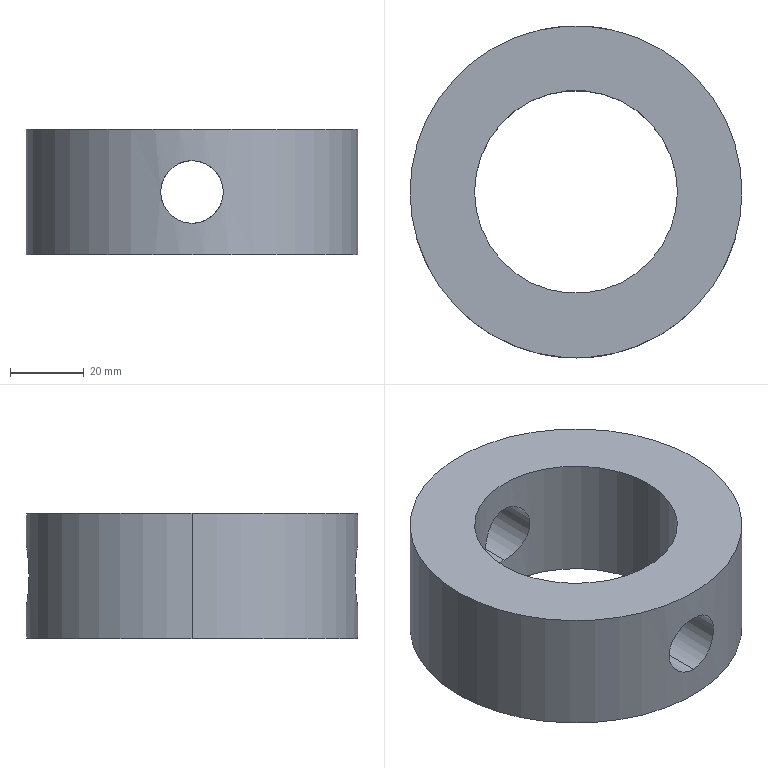Part | SolidWorks | features Extrusion 1, ICE 1 | 1 solid | 10 faces | box 90 x 90 x 34 mm | volume 127515 mm3 | cylinder 8 | plane 2 | commonest cylinder face diameters 17 x4 55 x2 90 x2
STEP:
#1=CARTESIAN_POINT('',(0.,-45.,8.5));
#2=VERTEX_POINT('',#1);
#3=CARTESIAN_POINT('',(0.,-45.,25.5));
#4=VERTEX_POINT('',#3);
#5=CARTESIAN_POINT('',(0.,-45.,8.5));
#6=CARTESIAN_POINT('',(-0.5553,-45.,8.5));
#7=CARTESIAN_POINT('',(-1.108,-44.99,8.554));
#8=CARTESIAN_POINT('',(-1.933,-44.959,8.718));
#9=CARTESIAN_POINT('',(-2.206,-44.947,8.786));
#10=CARTESIAN_POINT('',(-2.738,-44.917,8.948));
#11=CARTESIAN_POINT('',(-2.999,-44.901,9.042));
#12=CARTESIAN_POINT('',(-3.51,-44.864,9.254));
#13=CARTESIAN_POINT('',(-3.761,-44.843,9.372));
#14=CARTESIAN_POINT('',(-4.252,-44.799,9.635));
#15=CARTESIAN_POINT('',(-4.494,-44.776,9.78));
#16=CARTESIAN_POINT('',(-5.188,-44.702,10.244));
#17=CARTESIAN_POINT('',(-5.615,-44.65,10.595));
#18=CARTESIAN_POINT('',(-6.399,-44.544,11.378));
#19=CARTESIAN_POINT('',(-6.757,-44.491,11.814));
#20=CARTESIAN_POINT('',(-7.373,-44.393,12.734));
#21=CARTESIAN_POINT('',(-7.635,-44.348,13.222));
#22=CARTESIAN_POINT('',(-7.956,-44.291,13.995));
#23=CARTESIAN_POINT('',(-8.051,-44.274,14.26));
#24=CARTESIAN_POINT('',(-8.213,-44.244,14.793));
#25=CARTESIAN_POINT('',(-8.348,-44.219,15.331));
#26=CARTESIAN_POINT('',(-8.43,-44.203,15.88));
#27=CARTESIAN_POINT('',(-8.486,-44.193,16.434));
#28=CARTESIAN_POINT('',(-8.5,-44.19,16.715));
#29=CARTESIAN_POINT('',(-8.5,-44.19,17.557));
#30=CARTESIAN_POINT('',(-8.446,-44.201,18.109));
#31=CARTESIAN_POINT('',(-8.284,-44.231,18.926));
#32=CARTESIAN_POINT('',(-8.216,-44.244,19.196));
#33=CARTESIAN_POINT('',(-8.054,-44.274,19.732));
#34=CARTESIAN_POINT('',(-7.959,-44.291,19.997));
#35=CARTESIAN_POINT('',(-7.64,-44.347,20.767));
#36=CARTESIAN_POINT('',(-7.379,-44.392,21.255));
#37=CARTESIAN_POINT('',(-6.916,-44.466,21.949));
#38=CARTESIAN_POINT('',(-6.749,-44.491,22.175));
#39=CARTESIAN_POINT('',(-6.396,-44.544,22.606));
#40=CARTESIAN_POINT('',(-6.21,-44.57,22.811));
#41=CARTESIAN_POINT('',(-5.624,-44.649,23.397));
#42=CARTESIAN_POINT('',(-5.197,-44.701,23.75));
#43=CARTESIAN_POINT('',(-4.266,-44.8,24.373));
#44=CARTESIAN_POINT('',(-3.776,-44.844,24.635));
#45=CARTESIAN_POINT('',(-3.01,-44.9,24.954));
#46=CARTESIAN_POINT('',(-2.749,-44.917,25.048));
#47=CARTESIAN_POINT('',(-2.215,-44.946,25.211));
#48=CARTESIAN_POINT('',(-1.941,-44.959,25.28));
#49=CARTESIAN_POINT('',(-1.119,-44.989,25.445));
#50=CARTESIAN_POINT('',(-0.5628,-45.,25.5));
#51=CARTESIAN_POINT('',(0.,-45.,25.5));
#52=B_SPLINE_CURVE_WITH_KNOTS('',3,(#5,#6,#7,#8,#9,#10,#11,#12,#13,#14,#15,#16,#17,#18,#19,#20,#21,#22,#23,#24,#25,#26,#27,#28,#29,#30,#31,#32,#33,#34,#35,#36,#37,#38,#39,#40,#41,#42,#43,#44,#45,#46,#47,#48,#49,#50,#51),.UNSPECIFIED.,.F.,.F.,(4,2,2,2,2,2,2,2,2,2,1,2,2,2,2,2,2,2,2,2,2,2,2,4),(0.02663,0.0283,0.02913,0.02996,0.0308,0.03163,0.03329,0.03496,0.03662,0.03745,0.03828,0.03912,0.03995,0.04161,0.04245,0.04328,0.04494,0.04577,0.04661,0.04827,0.04993,0.05077,0.0516,0.05326),.UNSPECIFIED.);
#53=EDGE_CURVE('',#2,#4,#52,.T.);
#54=ORIENTED_EDGE('',*,*,#53,.F.);
#55=CARTESIAN_POINT('',(0.,-27.5,8.5));
#56=VERTEX_POINT('',#55);
#57=CARTESIAN_POINT('',(0.,-45.,8.5));
#58=DIRECTION('',(0.,1.,0.));
#59=VECTOR('',#58,1000.);
#60=LINE('',#57,#59);
#61=EDGE_CURVE('',#2,#56,#60,.T.);
#62=ORIENTED_EDGE('',*,*,#61,.T.);
#63=CARTESIAN_POINT('',(0.,-27.5,25.5));
#64=VERTEX_POINT('',#63);
#65=CARTESIAN_POINT('',(0.,-27.5,8.5));
#66=CARTESIAN_POINT('',(-0.2784,-27.5,8.5));
#67=CARTESIAN_POINT('',(-0.5567,-27.496,8.514));
#68=CARTESIAN_POINT('',(-1.113,-27.479,8.569));
#69=CARTESIAN_POINT('',(-1.392,-27.466,8.61));
#70=CARTESIAN_POINT('',(-2.219,-27.416,8.776));
#71=CARTESIAN_POINT('',(-2.751,-27.367,8.938));
#72=CARTESIAN_POINT('',(-3.776,-27.244,9.364));
#73=CARTESIAN_POINT('',(-4.273,-27.17,9.631));
#74=CARTESIAN_POINT('',(-5.192,-27.009,10.247));
#75=CARTESIAN_POINT('',(-5.618,-26.923,10.597));
#76=CARTESIAN_POINT('',(-6.206,-26.791,11.185));
#77=CARTESIAN_POINT('',(-6.394,-26.747,11.393));
#78=CARTESIAN_POINT('',(-6.746,-26.66,11.821));
#79=CARTESIAN_POINT('',(-6.91,-26.618,12.042));
#80=CARTESIAN_POINT('',(-7.37,-26.496,12.729));
#81=CARTESIAN_POINT('',(-7.633,-26.42,13.218));
#82=CARTESIAN_POINT('',(-8.063,-26.292,14.253));
#83=CARTESIAN_POINT('',(-8.225,-26.241,14.784));
#84=CARTESIAN_POINT('',(-8.389,-26.189,15.602));
#85=CARTESIAN_POINT('',(-8.43,-26.176,15.878));
#86=CARTESIAN_POINT('',(-8.486,-26.158,16.436));
#87=CARTESIAN_POINT('',(-8.5,-26.153,16.72));
#88=CARTESIAN_POINT('',(-8.5,-26.153,17.56));
#89=CARTESIAN_POINT('',(-8.445,-26.171,18.114));
#90=CARTESIAN_POINT('',(-8.281,-26.224,18.936));
#91=CARTESIAN_POINT('',(-8.212,-26.245,19.21));
#92=CARTESIAN_POINT('',(-8.049,-26.296,19.746));
#93=CARTESIAN_POINT('',(-7.955,-26.325,20.008));
#94=CARTESIAN_POINT('',(-7.636,-26.42,20.776));
#95=CARTESIAN_POINT('',(-7.374,-26.495,21.265));
#96=CARTESIAN_POINT('',(-6.753,-26.66,22.193));
#97=CARTESIAN_POINT('',(-6.402,-26.747,22.619));
#98=CARTESIAN_POINT('',(-5.818,-26.878,23.203));
#99=CARTESIAN_POINT('',(-5.613,-26.922,23.389));
#100=CARTESIAN_POINT('',(-5.184,-27.008,23.742));
#101=CARTESIAN_POINT('',(-4.959,-27.05,23.909));
#102=CARTESIAN_POINT('',(-4.269,-27.171,24.371));
#103=CARTESIAN_POINT('',(-3.782,-27.244,24.632));
#104=CARTESIAN_POINT('',(-3.013,-27.336,24.953));
#105=CARTESIAN_POINT('',(-2.749,-27.364,25.048));
#106=CARTESIAN_POINT('',(-2.212,-27.412,25.212));
#107=CARTESIAN_POINT('',(-1.941,-27.433,25.28));
#108=CARTESIAN_POINT('',(-1.121,-27.483,25.444));
#109=CARTESIAN_POINT('',(-0.5652,-27.5,25.5));
#110=CARTESIAN_POINT('',(0.,-27.5,25.5));
#111=B_SPLINE_CURVE_WITH_KNOTS('',3,(#65,#66,#67,#68,#69,#70,#71,#72,#73,#74,#75,#76,#77,#78,#79,#80,#81,#82,#83,#84,#85,#86,#87,#88,#89,#90,#91,#92,#93,#94,#95,#96,#97,#98,#99,#100,#101,#102,#103,#104,#105,#106,#107,#108,#109,#110),.UNSPECIFIED.,.F.,.F.,(4,2,2,2,2,2,2,2,2,2,2,2,2,2,2,2,2,2,2,2,2,2,4),(0.02674,0.02758,0.02841,0.03008,0.03175,0.03342,0.03426,0.03509,0.03676,0.03844,0.03927,0.04011,0.04178,0.04261,0.04345,0.04512,0.04679,0.04762,0.04846,0.05013,0.05097,0.0518,0.05347),.UNSPECIFIED.);
#112=EDGE_CURVE('',#56,#64,#111,.T.);
#113=ORIENTED_EDGE('',*,*,#112,.T.);
#114=CARTESIAN_POINT('',(0.,-45.,25.5));
#115=DIRECTION('',(0.,1.,0.));
#116=VECTOR('',#115,1000.);
#117=LINE('',#114,#116);
#118=EDGE_CURVE('',#4,#64,#117,.T.);
#119=ORIENTED_EDGE('',*,*,#118,.F.);
#120=EDGE_LOOP('',(#54,#62,#113,#119));
#121=FACE_OUTER_BOUND('',#120,.T.);
#122=CARTESIAN_POINT('',(0.,-45.,17.));
#123=DIRECTION('',(0.,1.,0.));
#124=DIRECTION('',(0.,0.,1.));
#125=AXIS2_PLACEMENT_3D('',#122,#123,#124);
#126=CYLINDRICAL_SURFACE('',#125,8.5);
#127=ADVANCED_FACE('',(#121),#126,.F.);
#128=CARTESIAN_POINT('',(0.,27.5,25.5));
#129=VERTEX_POINT('',#128);
#130=CARTESIAN_POINT('',(0.,27.5,8.5));
#131=VERTEX_POINT('',#130);
#132=CARTESIAN_POINT('',(0.,27.5,25.5));
#133=CARTESIAN_POINT('',(-0.5653,27.5,25.5));
#134=CARTESIAN_POINT('',(-1.121,27.483,25.444));
#135=CARTESIAN_POINT('',(-1.939,27.433,25.281));
#136=CARTESIAN_POINT('',(-2.209,27.412,25.213));
#137=CARTESIAN_POINT('',(-2.745,27.364,25.049));
#138=CARTESIAN_POINT('',(-3.011,27.336,24.954));
#139=CARTESIAN_POINT('',(-3.782,27.244,24.633));
#140=CARTESIAN_POINT('',(-4.269,27.171,24.371));
#141=CARTESIAN_POINT('',(-4.96,27.05,23.909));
#142=CARTESIAN_POINT('',(-5.185,27.008,23.741));
#143=CARTESIAN_POINT('',(-5.614,26.922,23.389));
#144=CARTESIAN_POINT('',(-5.818,26.878,23.203));
#145=CARTESIAN_POINT('',(-6.402,26.747,22.618));
#146=CARTESIAN_POINT('',(-6.753,26.66,22.193));
#147=CARTESIAN_POINT('',(-7.374,26.495,21.265));
#148=CARTESIAN_POINT('',(-7.635,26.42,20.776));
#149=CARTESIAN_POINT('',(-7.954,26.325,20.01));
#150=CARTESIAN_POINT('',(-8.048,26.296,19.749));
#151=CARTESIAN_POINT('',(-8.211,26.246,19.215));
#152=CARTESIAN_POINT('',(-8.28,26.224,18.94));
#153=CARTESIAN_POINT('',(-8.445,26.171,18.116));
#154=CARTESIAN_POINT('',(-8.5,26.153,17.562));
#155=CARTESIAN_POINT('',(-8.5,26.153,16.446));
#156=CARTESIAN_POINT('',(-8.444,26.172,15.878));
#157=CARTESIAN_POINT('',(-8.225,26.241,14.785));
#158=CARTESIAN_POINT('',(-8.064,26.292,14.254));
#159=CARTESIAN_POINT('',(-7.741,26.388,13.479));
#160=CARTESIAN_POINT('',(-7.621,26.423,13.225));
#161=CARTESIAN_POINT('',(-7.359,26.498,12.736));
#162=CARTESIAN_POINT('',(-7.216,26.537,12.5));
#163=CARTESIAN_POINT('',(-6.909,26.618,12.041));
#164=CARTESIAN_POINT('',(-6.744,26.661,11.819));
#165=CARTESIAN_POINT('',(-6.393,26.747,11.391));
#166=CARTESIAN_POINT('',(-6.204,26.792,11.183));
#167=CARTESIAN_POINT('',(-5.616,26.923,10.596));
#168=CARTESIAN_POINT('',(-5.191,27.01,10.246));
#169=CARTESIAN_POINT('',(-4.272,27.17,9.631));
#170=CARTESIAN_POINT('',(-3.774,27.245,9.364));
#171=CARTESIAN_POINT('',(-2.75,27.367,8.938));
#172=CARTESIAN_POINT('',(-2.22,27.416,8.776));
#173=CARTESIAN_POINT('',(-1.396,27.466,8.611));
#174=CARTESIAN_POINT('',(-1.115,27.479,8.569));
#175=CARTESIAN_POINT('',(-0.5572,27.496,8.514));
#176=CARTESIAN_POINT('',(-0.2785,27.5,8.5));
#177=CARTESIAN_POINT('',(0.,27.5,8.5));
#178=B_SPLINE_CURVE_WITH_KNOTS('',3,(#132,#133,#134,#135,#136,#137,#138,#139,#140,#141,#142,#143,#144,#145,#146,#147,#148,#149,#150,#151,#152,#153,#154,#155,#156,#157,#158,#159,#160,#161,#162,#163,#164,#165,#166,#167,#168,#169,#170,#171,#172,#173,#174,#175,#176,#177),.UNSPECIFIED.,.F.,.F.,(4,2,2,2,2,2,2,2,2,2,2,2,2,2,2,2,2,2,2,2,2,2,4),(0.,0.001671,0.002507,0.003342,0.005014,0.005849,0.006685,0.008356,0.01003,0.01086,0.0117,0.01337,0.01504,0.01671,0.01755,0.01838,0.01922,0.02005,0.02173,0.0234,0.02507,0.0259,0.02674),.UNSPECIFIED.);
#179=EDGE_CURVE('',#129,#131,#178,.T.);
#180=ORIENTED_EDGE('',*,*,#179,.T.);
#181=CARTESIAN_POINT('',(0.,45.,8.5));
#182=VERTEX_POINT('',#181);
#183=CARTESIAN_POINT('',(0.,-45.,8.5));
#184=DIRECTION('',(0.,1.,0.));
#185=VECTOR('',#184,1000.);
#186=LINE('',#183,#185);
#187=EDGE_CURVE('',#131,#182,#186,.T.);
#188=ORIENTED_EDGE('',*,*,#187,.T.);
#189=CARTESIAN_POINT('',(0.,45.,25.5));
#190=VERTEX_POINT('',#189);
#191=CARTESIAN_POINT('',(0.,45.,25.5));
#192=CARTESIAN_POINT('',(-0.563,45.,25.5));
#193=CARTESIAN_POINT('',(-1.116,44.989,25.445));
#194=CARTESIAN_POINT('',(-1.932,44.959,25.282));
#195=CARTESIAN_POINT('',(-2.202,44.947,25.215));
#196=CARTESIAN_POINT('',(-2.737,44.917,25.052));
#197=CARTESIAN_POINT('',(-3.002,44.9,24.957));
#198=CARTESIAN_POINT('',(-3.774,44.844,24.637));
#199=CARTESIAN_POINT('',(-4.262,44.8,24.375));
#200=CARTESIAN_POINT('',(-4.954,44.727,23.913));
#201=CARTESIAN_POINT('',(-5.179,44.701,23.746));
#202=CARTESIAN_POINT('',(-5.611,44.649,23.391));
#203=CARTESIAN_POINT('',(-5.816,44.623,23.205));
#204=CARTESIAN_POINT('',(-6.403,44.544,22.618));
#205=CARTESIAN_POINT('',(-6.754,44.491,22.191));
#206=CARTESIAN_POINT('',(-7.22,44.417,21.494));
#207=CARTESIAN_POINT('',(-7.365,44.393,21.253));
#208=CARTESIAN_POINT('',(-7.626,44.349,20.764));
#209=CARTESIAN_POINT('',(-7.745,44.329,20.513));
#210=CARTESIAN_POINT('',(-7.957,44.291,20.002));
#211=CARTESIAN_POINT('',(-8.051,44.274,19.741));
#212=CARTESIAN_POINT('',(-8.213,44.244,19.208));
#213=CARTESIAN_POINT('',(-8.282,44.231,18.935));
#214=CARTESIAN_POINT('',(-8.446,44.201,18.112));
#215=CARTESIAN_POINT('',(-8.5,44.19,17.559));
#216=CARTESIAN_POINT('',(-8.5,44.19,16.447));
#217=CARTESIAN_POINT('',(-8.445,44.201,15.883));
#218=CARTESIAN_POINT('',(-8.227,44.242,14.792));
#219=CARTESIAN_POINT('',(-8.066,44.272,14.261));
#220=CARTESIAN_POINT('',(-7.746,44.329,13.488));
#221=CARTESIAN_POINT('',(-7.625,44.349,13.233));
#222=CARTESIAN_POINT('',(-7.362,44.394,12.742));
#223=CARTESIAN_POINT('',(-7.219,44.417,12.505));
#224=CARTESIAN_POINT('',(-6.758,44.491,11.815));
#225=CARTESIAN_POINT('',(-6.405,44.544,11.385));
#226=CARTESIAN_POINT('',(-5.615,44.65,10.594));
#227=CARTESIAN_POINT('',(-5.187,44.702,10.243));
#228=CARTESIAN_POINT('',(-4.497,44.775,9.782));
#229=CARTESIAN_POINT('',(-4.259,44.799,9.639));
#230=CARTESIAN_POINT('',(-3.767,44.843,9.375));
#231=CARTESIAN_POINT('',(-3.513,44.863,9.255));
#232=CARTESIAN_POINT('',(-2.742,44.919,8.935));
#233=CARTESIAN_POINT('',(-2.212,44.949,8.774));
#234=CARTESIAN_POINT('',(-1.393,44.979,8.61));
#235=CARTESIAN_POINT('',(-1.114,44.987,8.569));
#236=CARTESIAN_POINT('',(-0.5561,44.997,8.514));
#237=CARTESIAN_POINT('',(-0.2777,45.,8.5));
#238=CARTESIAN_POINT('',(0.,45.,8.5));
#239=B_SPLINE_CURVE_WITH_KNOTS('',3,(#191,#192,#193,#194,#195,#196,#197,#198,#199,#200,#201,#202,#203,#204,#205,#206,#207,#208,#209,#210,#211,#212,#213,#214,#215,#216,#217,#218,#219,#220,#221,#222,#223,#224,#225,#226,#227,#228,#229,#230,#231,#232,#233,#234,#235,#236,#237,#238),.UNSPECIFIED.,.F.,.F.,(4,2,2,2,2,2,2,2,2,2,2,2,2,2,2,2,2,2,2,2,2,2,2,4),(0.,0.001665,0.002497,0.003329,0.004994,0.005826,0.006659,0.008323,0.009156,0.009988,0.01082,0.01165,0.01332,0.01498,0.01665,0.01748,0.01831,0.01998,0.02164,0.02247,0.02331,0.02497,0.0258,0.02663),.UNSPECIFIED.);
#240=EDGE_CURVE('',#190,#182,#239,.T.);
#241=ORIENTED_EDGE('',*,*,#240,.F.);
#242=CARTESIAN_POINT('',(0.,-45.,25.5));
#243=DIRECTION('',(0.,1.,0.));
#244=VECTOR('',#243,1000.);
#245=LINE('',#242,#244);
#246=EDGE_CURVE('',#129,#190,#245,.T.);
#247=ORIENTED_EDGE('',*,*,#246,.F.);
#248=EDGE_LOOP('',(#180,#188,#241,#247));
#249=FACE_OUTER_BOUND('',#248,.T.);
#250=CARTESIAN_POINT('',(0.,-45.,17.));
#251=DIRECTION('',(0.,1.,0.));
#252=DIRECTION('',(0.,0.,1.));
#253=AXIS2_PLACEMENT_3D('',#250,#251,#252);
#254=CYLINDRICAL_SURFACE('',#253,8.5);
#255=ADVANCED_FACE('',(#249),#254,.F.);
#256=CARTESIAN_POINT('',(0.,-27.5,25.5));
#257=CARTESIAN_POINT('',(0.5653,-27.5,25.5));
#258=CARTESIAN_POINT('',(1.121,-27.483,25.444));
#259=CARTESIAN_POINT('',(1.939,-27.433,25.281));
#260=CARTESIAN_POINT('',(2.209,-27.412,25.213));
#261=CARTESIAN_POINT('',(2.745,-27.364,25.049));
#262=CARTESIAN_POINT('',(3.011,-27.336,24.954));
#263=CARTESIAN_POINT('',(3.782,-27.244,24.633));
#264=CARTESIAN_POINT('',(4.269,-27.171,24.371));
#265=CARTESIAN_POINT('',(4.96,-27.05,23.909));
#266=CARTESIAN_POINT('',(5.185,-27.008,23.741));
#267=CARTESIAN_POINT('',(5.614,-26.922,23.389));
#268=CARTESIAN_POINT('',(5.818,-26.878,23.203));
#269=CARTESIAN_POINT('',(6.402,-26.747,22.618));
#270=CARTESIAN_POINT('',(6.753,-26.66,22.193));
#271=CARTESIAN_POINT('',(7.374,-26.495,21.265));
#272=CARTESIAN_POINT('',(7.635,-26.42,20.776));
#273=CARTESIAN_POINT('',(7.954,-26.325,20.01));
#274=CARTESIAN_POINT('',(8.048,-26.296,19.749));
#275=CARTESIAN_POINT('',(8.211,-26.246,19.215));
#276=CARTESIAN_POINT('',(8.28,-26.224,18.94));
#277=CARTESIAN_POINT('',(8.445,-26.171,18.116));
#278=CARTESIAN_POINT('',(8.5,-26.153,17.562));
#279=CARTESIAN_POINT('',(8.5,-26.153,16.446));
#280=CARTESIAN_POINT('',(8.444,-26.172,15.878));
#281=CARTESIAN_POINT('',(8.225,-26.241,14.785));
#282=CARTESIAN_POINT('',(8.064,-26.292,14.254));
#283=CARTESIAN_POINT('',(7.741,-26.388,13.479));
#284=CARTESIAN_POINT('',(7.621,-26.423,13.225));
#285=CARTESIAN_POINT('',(7.359,-26.498,12.736));
#286=CARTESIAN_POINT('',(7.216,-26.537,12.5));
#287=CARTESIAN_POINT('',(6.909,-26.618,12.041));
#288=CARTESIAN_POINT('',(6.744,-26.661,11.819));
#289=CARTESIAN_POINT('',(6.393,-26.747,11.391));
#290=CARTESIAN_POINT('',(6.204,-26.792,11.183));
#291=CARTESIAN_POINT('',(5.616,-26.923,10.596));
#292=CARTESIAN_POINT('',(5.191,-27.01,10.246));
#293=CARTESIAN_POINT('',(4.272,-27.17,9.631));
#294=CARTESIAN_POINT('',(3.774,-27.245,9.364));
#295=CARTESIAN_POINT('',(2.75,-27.367,8.938));
#296=CARTESIAN_POINT('',(2.22,-27.416,8.776));
#297=CARTESIAN_POINT('',(1.396,-27.466,8.611));
#298=CARTESIAN_POINT('',(1.115,-27.479,8.569));
#299=CARTESIAN_POINT('',(0.5572,-27.496,8.514));
#300=CARTESIAN_POINT('',(0.2785,-27.5,8.5));
#301=CARTESIAN_POINT('',(0.,-27.5,8.5));
#302=B_SPLINE_CURVE_WITH_KNOTS('',3,(#256,#257,#258,#259,#260,#261,#262,#263,#264,#265,#266,#267,#268,#269,#270,#271,#272,#273,#274,#275,#276,#277,#278,#279,#280,#281,#282,#283,#284,#285,#286,#287,#288,#289,#290,#291,#292,#293,#294,#295,#296,#297,#298,#299,#300,#301),.UNSPECIFIED.,.F.,.F.,(4,2,2,2,2,2,2,2,2,2,2,2,2,2,2,2,2,2,2,2,2,2,4),(0.,0.001671,0.002507,0.003342,0.005014,0.005849,0.006685,0.008356,0.01003,0.01086,0.0117,0.01337,0.01504,0.01671,0.01755,0.01838,0.01922,0.02005,0.02173,0.0234,0.02507,0.0259,0.02674),.UNSPECIFIED.);
#303=EDGE_CURVE('',#64,#56,#302,.T.);
#304=ORIENTED_EDGE('',*,*,#303,.F.);
#305=ORIENTED_EDGE('',*,*,#112,.F.);
#306=EDGE_LOOP('',(#304,#305));
#307=FACE_BOUND('',#306,.T.);
#308=CARTESIAN_POINT('',(-27.5,0.,34.));
#309=VERTEX_POINT('',#308);
#310=CARTESIAN_POINT('',(27.5,0.,34.));
#311=VERTEX_POINT('',#310);
#312=CARTESIAN_POINT('',(0.,0.,34.));
#313=DIRECTION('',(0.,0.,1.));
#314=DIRECTION('',(1.,0.,0.));
#315=AXIS2_PLACEMENT_3D('',#312,#313,#314);
#316=CIRCLE('',#315,27.5);
#317=EDGE_CURVE('',#309,#311,#316,.T.);
#318=ORIENTED_EDGE('',*,*,#317,.T.);
#319=CARTESIAN_POINT('',(27.5,0.,0.));
#320=VERTEX_POINT('',#319);
#321=CARTESIAN_POINT('',(27.5,0.,34.));
#322=DIRECTION('',(0.,0.,-1.));
#323=VECTOR('',#322,1000.);
#324=LINE('',#321,#323);
#325=EDGE_CURVE('',#311,#320,#324,.T.);
#326=ORIENTED_EDGE('',*,*,#325,.T.);
#327=CARTESIAN_POINT('',(-27.5,0.,0.));
#328=VERTEX_POINT('',#327);
#329=CARTESIAN_POINT('',(0.,0.,0.));
#330=DIRECTION('',(0.,0.,1.));
#331=DIRECTION('',(1.,0.,0.));
#332=AXIS2_PLACEMENT_3D('',#329,#330,#331);
#333=CIRCLE('',#332,27.5);
#334=EDGE_CURVE('',#328,#320,#333,.T.);
#335=ORIENTED_EDGE('',*,*,#334,.F.);
#336=CARTESIAN_POINT('',(-27.5,0.,34.));
#337=DIRECTION('',(0.,0.,-1.));
#338=VECTOR('',#337,1000.);
#339=LINE('',#336,#338);
#340=EDGE_CURVE('',#309,#328,#339,.T.);
#341=ORIENTED_EDGE('',*,*,#340,.F.);
#342=EDGE_LOOP('',(#318,#326,#335,#341));
#343=FACE_OUTER_BOUND('',#342,.T.);
#344=CARTESIAN_POINT('',(0.,0.,34.));
#345=DIRECTION('',(0.,0.,-1.));
#346=DIRECTION('',(-1.,0.,0.));
#347=AXIS2_PLACEMENT_3D('',#344,#345,#346);
#348=CYLINDRICAL_SURFACE('',#347,27.5);
#349=ADVANCED_FACE('',(#307,#343),#348,.F.);
#350=ORIENTED_EDGE('',*,*,#240,.T.);
#351=CARTESIAN_POINT('',(0.,45.,8.5));
#352=CARTESIAN_POINT('',(0.5553,45.,8.5));
#353=CARTESIAN_POINT('',(1.108,44.99,8.554));
#354=CARTESIAN_POINT('',(1.933,44.959,8.718));
#355=CARTESIAN_POINT('',(2.206,44.947,8.786));
#356=CARTESIAN_POINT('',(2.738,44.917,8.948));
#357=CARTESIAN_POINT('',(2.999,44.901,9.042));
#358=CARTESIAN_POINT('',(3.51,44.864,9.254));
#359=CARTESIAN_POINT('',(3.761,44.843,9.372));
#360=CARTESIAN_POINT('',(4.252,44.799,9.635));
#361=CARTESIAN_POINT('',(4.494,44.776,9.78));
#362=CARTESIAN_POINT('',(5.188,44.702,10.244));
#363=CARTESIAN_POINT('',(5.615,44.65,10.595));
#364=CARTESIAN_POINT('',(6.399,44.544,11.378));
#365=CARTESIAN_POINT('',(6.757,44.491,11.814));
#366=CARTESIAN_POINT('',(7.373,44.393,12.734));
#367=CARTESIAN_POINT('',(7.635,44.348,13.222));
#368=CARTESIAN_POINT('',(7.956,44.291,13.995));
#369=CARTESIAN_POINT('',(8.051,44.274,14.26));
#370=CARTESIAN_POINT('',(8.213,44.244,14.793));
#371=CARTESIAN_POINT('',(8.348,44.219,15.331));
#372=CARTESIAN_POINT('',(8.43,44.203,15.88));
#373=CARTESIAN_POINT('',(8.486,44.193,16.434));
#374=CARTESIAN_POINT('',(8.5,44.19,16.715));
#375=CARTESIAN_POINT('',(8.5,44.19,17.557));
#376=CARTESIAN_POINT('',(8.446,44.201,18.109));
#377=CARTESIAN_POINT('',(8.284,44.231,18.926));
#378=CARTESIAN_POINT('',(8.216,44.244,19.196));
#379=CARTESIAN_POINT('',(8.054,44.274,19.732));
#380=CARTESIAN_POINT('',(7.959,44.291,19.997));
#381=CARTESIAN_POINT('',(7.64,44.347,20.767));
#382=CARTESIAN_POINT('',(7.379,44.392,21.255));
#383=CARTESIAN_POINT('',(6.916,44.466,21.949));
#384=CARTESIAN_POINT('',(6.749,44.491,22.175));
#385=CARTESIAN_POINT('',(6.396,44.544,22.606));
#386=CARTESIAN_POINT('',(6.21,44.57,22.811));
#387=CARTESIAN_POINT('',(5.624,44.649,23.397));
#388=CARTESIAN_POINT('',(5.197,44.701,23.75));
#389=CARTESIAN_POINT('',(4.266,44.8,24.373));
#390=CARTESIAN_POINT('',(3.776,44.844,24.635));
#391=CARTESIAN_POINT('',(3.01,44.9,24.954));
#392=CARTESIAN_POINT('',(2.749,44.917,25.048));
#393=CARTESIAN_POINT('',(2.215,44.946,25.211));
#394=CARTESIAN_POINT('',(1.941,44.959,25.28));
#395=CARTESIAN_POINT('',(1.119,44.989,25.445));
#396=CARTESIAN_POINT('',(0.5628,45.,25.5));
#397=CARTESIAN_POINT('',(0.,45.,25.5));
#398=B_SPLINE_CURVE_WITH_KNOTS('',3,(#351,#352,#353,#354,#355,#356,#357,#358,#359,#360,#361,#362,#363,#364,#365,#366,#367,#368,#369,#370,#371,#372,#373,#374,#375,#376,#377,#378,#379,#380,#381,#382,#383,#384,#385,#386,#387,#388,#389,#390,#391,#392,#393,#394,#395,#396,#397),.UNSPECIFIED.,.F.,.F.,(4,2,2,2,2,2,2,2,2,2,1,2,2,2,2,2,2,2,2,2,2,2,2,4),(0.02663,0.0283,0.02913,0.02996,0.0308,0.03163,0.03329,0.03496,0.03662,0.03745,0.03828,0.03912,0.03995,0.04161,0.04245,0.04328,0.04494,0.04577,0.04661,0.04827,0.04993,0.05077,0.0516,0.05326),.UNSPECIFIED.);
#399=EDGE_CURVE('',#182,#190,#398,.T.);
#400=ORIENTED_EDGE('',*,*,#399,.T.);
#401=EDGE_LOOP('',(#350,#400));
#402=FACE_BOUND('',#401,.T.);
#403=CARTESIAN_POINT('',(45.,0.,34.));
#404=VERTEX_POINT('',#403);
#405=CARTESIAN_POINT('',(-45.,0.,34.));
#406=VERTEX_POINT('',#405);
#407=CARTESIAN_POINT('',(0.,0.,34.));
#408=DIRECTION('',(0.,0.,1.));
#409=DIRECTION('',(1.,0.,0.));
#410=AXIS2_PLACEMENT_3D('',#407,#408,#409);
#411=CIRCLE('',#410,45.);
#412=EDGE_CURVE('',#404,#406,#411,.T.);
#413=ORIENTED_EDGE('',*,*,#412,.F.);
#414=CARTESIAN_POINT('',(45.,0.,0.));
#415=VERTEX_POINT('',#414);
#416=CARTESIAN_POINT('',(45.,0.,34.));
#417=DIRECTION('',(0.,0.,-1.));
#418=VECTOR('',#417,1000.);
#419=LINE('',#416,#418);
#420=EDGE_CURVE('',#404,#415,#419,.T.);
#421=ORIENTED_EDGE('',*,*,#420,.T.);
#422=CARTESIAN_POINT('',(-45.,0.,0.));
#423=VERTEX_POINT('',#422);
#424=CARTESIAN_POINT('',(0.,0.,0.));
#425=DIRECTION('',(0.,0.,1.));
#426=DIRECTION('',(1.,0.,0.));
#427=AXIS2_PLACEMENT_3D('',#424,#425,#426);
#428=CIRCLE('',#427,45.);
#429=EDGE_CURVE('',#415,#423,#428,.T.);
#430=ORIENTED_EDGE('',*,*,#429,.T.);
#431=CARTESIAN_POINT('',(-45.,0.,34.));
#432=DIRECTION('',(0.,0.,-1.));
#433=VECTOR('',#432,1000.);
#434=LINE('',#431,#433);
#435=EDGE_CURVE('',#406,#423,#434,.T.);
#436=ORIENTED_EDGE('',*,*,#435,.F.);
#437=EDGE_LOOP('',(#413,#421,#430,#436));
#438=FACE_OUTER_BOUND('',#437,.T.);
#439=CARTESIAN_POINT('',(0.,0.,34.));
#440=DIRECTION('',(0.,0.,-1.));
#441=DIRECTION('',(-1.,0.,0.));
#442=AXIS2_PLACEMENT_3D('',#439,#440,#441);
#443=CYLINDRICAL_SURFACE('',#442,45.);
#444=ADVANCED_FACE('',(#402,#438),#443,.T.);
#445=CARTESIAN_POINT('',(0.,0.,34.));
#446=DIRECTION('',(0.,0.,1.));
#447=DIRECTION('',(1.,0.,0.));
#448=AXIS2_PLACEMENT_3D('',#445,#446,#447);
#449=CIRCLE('',#448,45.);
#450=EDGE_CURVE('',#406,#404,#449,.T.);
#451=ORIENTED_EDGE('',*,*,#450,.T.);
#452=ORIENTED_EDGE('',*,*,#412,.T.);
#453=EDGE_LOOP('',(#451,#452));
#454=FACE_OUTER_BOUND('',#453,.T.);
#455=ORIENTED_EDGE('',*,*,#317,.F.);
#456=CARTESIAN_POINT('',(0.,0.,34.));
#457=DIRECTION('',(0.,0.,1.));
#458=DIRECTION('',(1.,0.,0.));
#459=AXIS2_PLACEMENT_3D('',#456,#457,#458);
#460=CIRCLE('',#459,27.5);
#461=EDGE_CURVE('',#311,#309,#460,.T.);
#462=ORIENTED_EDGE('',*,*,#461,.F.);
#463=EDGE_LOOP('',(#455,#462));
#464=FACE_BOUND('',#463,.T.);
#465=CARTESIAN_POINT('',(0.,0.,34.));
#466=DIRECTION('',(0.,0.,1.));
#467=DIRECTION('',(1.,0.,0.));
#468=AXIS2_PLACEMENT_3D('',#465,#466,#467);
#469=PLANE('',#468);
#470=ADVANCED_FACE('',(#454,#464),#469,.T.);
#471=CARTESIAN_POINT('',(0.,0.,0.));
#472=DIRECTION('',(0.,0.,1.));
#473=DIRECTION('',(1.,0.,0.));
#474=AXIS2_PLACEMENT_3D('',#471,#472,#473);
#475=CIRCLE('',#474,45.);
#476=EDGE_CURVE('',#423,#415,#475,.T.);
#477=ORIENTED_EDGE('',*,*,#476,.F.);
#478=ORIENTED_EDGE('',*,*,#429,.F.);
#479=EDGE_LOOP('',(#477,#478));
#480=FACE_OUTER_BOUND('',#479,.T.);
#481=ORIENTED_EDGE('',*,*,#334,.T.);
#482=CARTESIAN_POINT('',(0.,0.,0.));
#483=DIRECTION('',(0.,0.,1.));
#484=DIRECTION('',(1.,0.,0.));
#485=AXIS2_PLACEMENT_3D('',#482,#483,#484);
#486=CIRCLE('',#485,27.5);
#487=EDGE_CURVE('',#320,#328,#486,.T.);
#488=ORIENTED_EDGE('',*,*,#487,.T.);
#489=EDGE_LOOP('',(#481,#488));
#490=FACE_BOUND('',#489,.T.);
#491=CARTESIAN_POINT('',(0.,0.,0.));
#492=DIRECTION('',(0.,0.,1.));
#493=DIRECTION('',(1.,0.,0.));
#494=AXIS2_PLACEMENT_3D('',#491,#492,#493);
#495=PLANE('',#494);
#496=ADVANCED_FACE('',(#480,#490),#495,.F.);
#497=ORIENTED_EDGE('',*,*,#420,.F.);
#498=ORIENTED_EDGE('',*,*,#450,.F.);
#499=ORIENTED_EDGE('',*,*,#435,.T.);
#500=ORIENTED_EDGE('',*,*,#476,.T.);
#501=EDGE_LOOP('',(#497,#498,#499,#500));
#502=FACE_OUTER_BOUND('',#501,.T.);
#503=CARTESIAN_POINT('',(0.,-45.,25.5));
#504=CARTESIAN_POINT('',(0.563,-45.,25.5));
#505=CARTESIAN_POINT('',(1.116,-44.989,25.445));
#506=CARTESIAN_POINT('',(1.932,-44.959,25.282));
#507=CARTESIAN_POINT('',(2.202,-44.947,25.215));
#508=CARTESIAN_POINT('',(2.737,-44.917,25.052));
#509=CARTESIAN_POINT('',(3.002,-44.9,24.957));
#510=CARTESIAN_POINT('',(3.774,-44.844,24.637));
#511=CARTESIAN_POINT('',(4.262,-44.8,24.375));
#512=CARTESIAN_POINT('',(4.954,-44.727,23.913));
#513=CARTESIAN_POINT('',(5.179,-44.701,23.746));
#514=CARTESIAN_POINT('',(5.611,-44.649,23.391));
#515=CARTESIAN_POINT('',(5.816,-44.623,23.205));
#516=CARTESIAN_POINT('',(6.403,-44.544,22.618));
#517=CARTESIAN_POINT('',(6.754,-44.491,22.191));
#518=CARTESIAN_POINT('',(7.22,-44.417,21.494));
#519=CARTESIAN_POINT('',(7.365,-44.393,21.253));
#520=CARTESIAN_POINT('',(7.626,-44.349,20.764));
#521=CARTESIAN_POINT('',(7.745,-44.329,20.513));
#522=CARTESIAN_POINT('',(7.957,-44.291,20.002));
#523=CARTESIAN_POINT('',(8.051,-44.274,19.741));
#524=CARTESIAN_POINT('',(8.213,-44.244,19.208));
#525=CARTESIAN_POINT('',(8.282,-44.231,18.935));
#526=CARTESIAN_POINT('',(8.446,-44.201,18.112));
#527=CARTESIAN_POINT('',(8.5,-44.19,17.559));
#528=CARTESIAN_POINT('',(8.5,-44.19,16.447));
#529=CARTESIAN_POINT('',(8.445,-44.201,15.883));
#530=CARTESIAN_POINT('',(8.227,-44.242,14.792));
#531=CARTESIAN_POINT('',(8.066,-44.272,14.261));
#532=CARTESIAN_POINT('',(7.746,-44.329,13.488));
#533=CARTESIAN_POINT('',(7.625,-44.349,13.233));
#534=CARTESIAN_POINT('',(7.362,-44.394,12.742));
#535=CARTESIAN_POINT('',(7.219,-44.417,12.505));
#536=CARTESIAN_POINT('',(6.758,-44.491,11.815));
#537=CARTESIAN_POINT('',(6.405,-44.544,11.385));
#538=CARTESIAN_POINT('',(5.615,-44.65,10.594));
#539=CARTESIAN_POINT('',(5.187,-44.702,10.243));
#540=CARTESIAN_POINT('',(4.497,-44.775,9.782));
#541=CARTESIAN_POINT('',(4.259,-44.799,9.639));
#542=CARTESIAN_POINT('',(3.767,-44.843,9.375));
#543=CARTESIAN_POINT('',(3.513,-44.863,9.255));
#544=CARTESIAN_POINT('',(2.742,-44.919,8.935));
#545=CARTESIAN_POINT('',(2.212,-44.949,8.774));
#546=CARTESIAN_POINT('',(1.393,-44.979,8.61));
#547=CARTESIAN_POINT('',(1.114,-44.987,8.569));
#548=CARTESIAN_POINT('',(0.5561,-44.997,8.514));
#549=CARTESIAN_POINT('',(0.2777,-45.,8.5));
#550=CARTESIAN_POINT('',(0.,-45.,8.5));
#551=B_SPLINE_CURVE_WITH_KNOTS('',3,(#503,#504,#505,#506,#507,#508,#509,#510,#511,#512,#513,#514,#515,#516,#517,#518,#519,#520,#521,#522,#523,#524,#525,#526,#527,#528,#529,#530,#531,#532,#533,#534,#535,#536,#537,#538,#539,#540,#541,#542,#543,#544,#545,#546,#547,#548,#549,#550),.UNSPECIFIED.,.F.,.F.,(4,2,2,2,2,2,2,2,2,2,2,2,2,2,2,2,2,2,2,2,2,2,2,4),(0.,0.001665,0.002497,0.003329,0.004994,0.005826,0.006659,0.008323,0.009156,0.009988,0.01082,0.01165,0.01332,0.01498,0.01665,0.01748,0.01831,0.01998,0.02164,0.02247,0.02331,0.02497,0.0258,0.02663),.UNSPECIFIED.);
#552=EDGE_CURVE('',#4,#2,#551,.T.);
#553=ORIENTED_EDGE('',*,*,#552,.T.);
#554=ORIENTED_EDGE('',*,*,#53,.T.);
#555=EDGE_LOOP('',(#553,#554));
#556=FACE_BOUND('',#555,.T.);
#557=CARTESIAN_POINT('',(0.,0.,34.));
#558=DIRECTION('',(0.,0.,-1.));
#559=DIRECTION('',(-1.,0.,0.));
#560=AXIS2_PLACEMENT_3D('',#557,#558,#559);
#561=CYLINDRICAL_SURFACE('',#560,45.);
#562=ADVANCED_FACE('',(#502,#556),#561,.T.);
#563=ORIENTED_EDGE('',*,*,#325,.F.);
#564=ORIENTED_EDGE('',*,*,#461,.T.);
#565=ORIENTED_EDGE('',*,*,#340,.T.);
#566=ORIENTED_EDGE('',*,*,#487,.F.);
#567=EDGE_LOOP('',(#563,#564,#565,#566));
#568=FACE_OUTER_BOUND('',#567,.T.);
#569=ORIENTED_EDGE('',*,*,#179,.F.);
#570=CARTESIAN_POINT('',(0.,27.5,8.5));
#571=CARTESIAN_POINT('',(0.2784,27.5,8.5));
#572=CARTESIAN_POINT('',(0.5567,27.496,8.514));
#573=CARTESIAN_POINT('',(1.113,27.479,8.569));
#574=CARTESIAN_POINT('',(1.392,27.466,8.61));
#575=CARTESIAN_POINT('',(2.219,27.416,8.776));
#576=CARTESIAN_POINT('',(2.751,27.367,8.938));
#577=CARTESIAN_POINT('',(3.776,27.244,9.364));
#578=CARTESIAN_POINT('',(4.273,27.17,9.631));
#579=CARTESIAN_POINT('',(5.192,27.009,10.247));
#580=CARTESIAN_POINT('',(5.618,26.923,10.597));
#581=CARTESIAN_POINT('',(6.206,26.791,11.185));
#582=CARTESIAN_POINT('',(6.394,26.747,11.393));
#583=CARTESIAN_POINT('',(6.746,26.66,11.821));
#584=CARTESIAN_POINT('',(6.91,26.618,12.042));
#585=CARTESIAN_POINT('',(7.37,26.496,12.729));
#586=CARTESIAN_POINT('',(7.633,26.42,13.218));
#587=CARTESIAN_POINT('',(8.063,26.292,14.253));
#588=CARTESIAN_POINT('',(8.225,26.241,14.784));
#589=CARTESIAN_POINT('',(8.389,26.189,15.602));
#590=CARTESIAN_POINT('',(8.43,26.176,15.878));
#591=CARTESIAN_POINT('',(8.486,26.158,16.436));
#592=CARTESIAN_POINT('',(8.5,26.153,16.72));
#593=CARTESIAN_POINT('',(8.5,26.153,17.56));
#594=CARTESIAN_POINT('',(8.445,26.171,18.114));
#595=CARTESIAN_POINT('',(8.281,26.224,18.936));
#596=CARTESIAN_POINT('',(8.212,26.245,19.21));
#597=CARTESIAN_POINT('',(8.049,26.296,19.746));
#598=CARTESIAN_POINT('',(7.955,26.325,20.008));
#599=CARTESIAN_POINT('',(7.636,26.42,20.776));
#600=CARTESIAN_POINT('',(7.374,26.495,21.265));
#601=CARTESIAN_POINT('',(6.753,26.66,22.193));
#602=CARTESIAN_POINT('',(6.402,26.747,22.619));
#603=CARTESIAN_POINT('',(5.818,26.878,23.203));
#604=CARTESIAN_POINT('',(5.613,26.922,23.389));
#605=CARTESIAN_POINT('',(5.184,27.008,23.742));
#606=CARTESIAN_POINT('',(4.959,27.05,23.909));
#607=CARTESIAN_POINT('',(4.269,27.171,24.371));
#608=CARTESIAN_POINT('',(3.782,27.244,24.632));
#609=CARTESIAN_POINT('',(3.013,27.336,24.953));
#610=CARTESIAN_POINT('',(2.749,27.364,25.048));
#611=CARTESIAN_POINT('',(2.212,27.412,25.212));
#612=CARTESIAN_POINT('',(1.941,27.433,25.28));
#613=CARTESIAN_POINT('',(1.121,27.483,25.444));
#614=CARTESIAN_POINT('',(0.5652,27.5,25.5));
#615=CARTESIAN_POINT('',(0.,27.5,25.5));
#616=B_SPLINE_CURVE_WITH_KNOTS('',3,(#570,#571,#572,#573,#574,#575,#576,#577,#578,#579,#580,#581,#582,#583,#584,#585,#586,#587,#588,#589,#590,#591,#592,#593,#594,#595,#596,#597,#598,#599,#600,#601,#602,#603,#604,#605,#606,#607,#608,#609,#610,#611,#612,#613,#614,#615),.UNSPECIFIED.,.F.,.F.,(4,2,2,2,2,2,2,2,2,2,2,2,2,2,2,2,2,2,2,2,2,2,4),(0.02674,0.02758,0.02841,0.03008,0.03175,0.03342,0.03426,0.03509,0.03676,0.03844,0.03927,0.04011,0.04178,0.04261,0.04345,0.04512,0.04679,0.04762,0.04846,0.05013,0.05097,0.0518,0.05347),.UNSPECIFIED.);
#617=EDGE_CURVE('',#131,#129,#616,.T.);
#618=ORIENTED_EDGE('',*,*,#617,.F.);
#619=EDGE_LOOP('',(#569,#618));
#620=FACE_BOUND('',#619,.T.);
#621=CARTESIAN_POINT('',(0.,0.,34.));
#622=DIRECTION('',(0.,0.,-1.));
#623=DIRECTION('',(-1.,0.,0.));
#624=AXIS2_PLACEMENT_3D('',#621,#622,#623);
#625=CYLINDRICAL_SURFACE('',#624,27.5);
#626=ADVANCED_FACE('',(#568,#620),#625,.F.);
#627=ORIENTED_EDGE('',*,*,#187,.F.);
#628=ORIENTED_EDGE('',*,*,#617,.T.);
#629=ORIENTED_EDGE('',*,*,#246,.T.);
#630=ORIENTED_EDGE('',*,*,#399,.F.);
#631=EDGE_LOOP('',(#627,#628,#629,#630));
#632=FACE_OUTER_BOUND('',#631,.T.);
#633=CARTESIAN_POINT('',(0.,-45.,17.));
#634=DIRECTION('',(0.,1.,0.));
#635=DIRECTION('',(0.,0.,1.));
#636=AXIS2_PLACEMENT_3D('',#633,#634,#635);
#637=CYLINDRICAL_SURFACE('',#636,8.5);
#638=ADVANCED_FACE('',(#632),#637,.F.);
#639=ORIENTED_EDGE('',*,*,#61,.F.);
#640=ORIENTED_EDGE('',*,*,#552,.F.);
#641=ORIENTED_EDGE('',*,*,#118,.T.);
#642=ORIENTED_EDGE('',*,*,#303,.T.);
#643=EDGE_LOOP('',(#639,#640,#641,#642));
#644=FACE_OUTER_BOUND('',#643,.T.);
#645=CARTESIAN_POINT('',(0.,-45.,17.));
#646=DIRECTION('',(0.,1.,0.));
#647=DIRECTION('',(0.,0.,1.));
#648=AXIS2_PLACEMENT_3D('',#645,#646,#647);
#649=CYLINDRICAL_SURFACE('',#648,8.5);
#650=ADVANCED_FACE('',(#644),#649,.F.);
#651=CLOSED_SHELL('',(#127,#255,#349,#444,#470,#496,#562,#626,#638,#650));
#652=MANIFOLD_SOLID_BREP('',#651);
#653=CARTESIAN_POINT('',(0.,0.,0.));
#654=DIRECTION('',(0.,0.,1.));
#655=DIRECTION('',(1.,0.,0.));
#656=AXIS2_PLACEMENT_3D('',#653,#654,#655);
#657=(LENGTH_UNIT()NAMED_UNIT(*)SI_UNIT(.MILLI.,.METRE.));
#658=UNCERTAINTY_MEASURE_WITH_UNIT(LENGTH_MEASURE(0.00001),#657,'','');
#659=(NAMED_UNIT(*)PLANE_ANGLE_UNIT()SI_UNIT($,.RADIAN.));
#660=(NAMED_UNIT(*)SI_UNIT($,.STERADIAN.)SOLID_ANGLE_UNIT());
#661=(GEOMETRIC_REPRESENTATION_CONTEXT(3)GLOBAL_UNCERTAINTY_ASSIGNED_CONTEXT((#658))GLOBAL_UNIT_ASSIGNED_CONTEXT((#657,#659,#660))REPRESENTATION_CONTEXT('',''));
#662=ADVANCED_BREP_SHAPE_REPRESENTATION('',(#652,#656),#661);